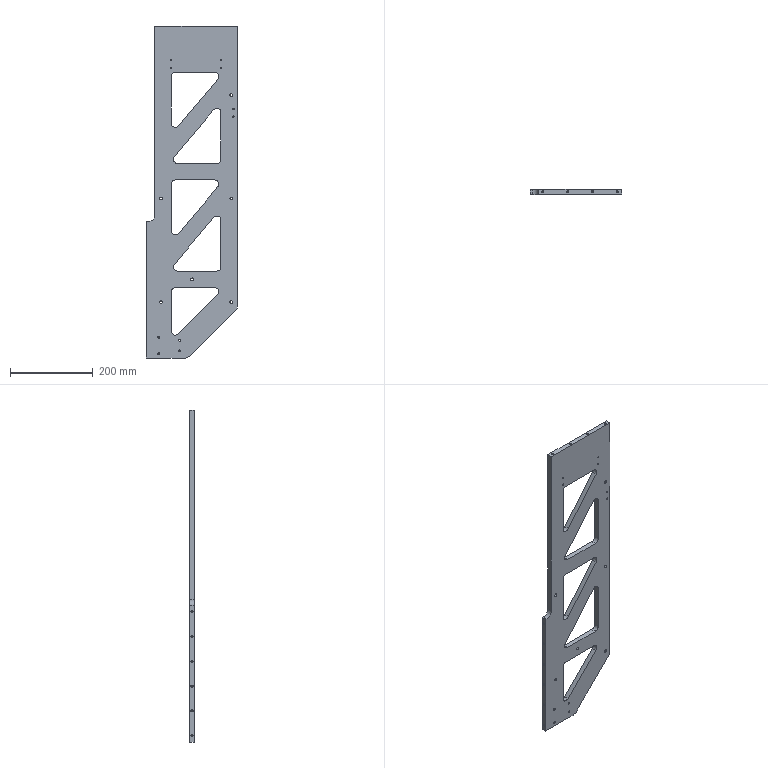Part | SolidWorks | features HoleWzd 8, ICE 2, Chamfer 1, Extrusion 1, Fillet 1 | 1 solid | 116 faces | box 220 x 12 x 802 mm | volume 1372017 mm3 | cylinder 72 | plane 24 | cone 20 | commonest cylinder face diameters 5 x24 20 x17 3.3 x12 6.6 x12 4.2 x4 30 x3